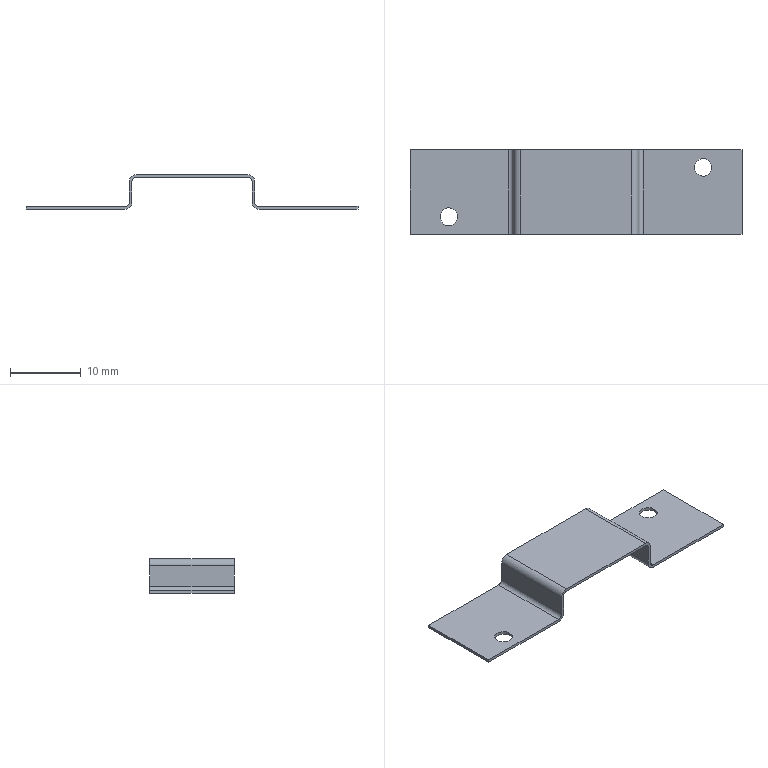Part | STEP file | ZXW722-L-04 | 1 solid | 26 faces | box 47 x 12 x 4.9 mm | volume 258.28 mm3 | plane 14 | cylinder 12 | commonest cylinder face diameters 1.2 x4 2 x4 2.5 x4
STEP:
#1=CARTESIAN_POINT('',(0.,0.,0.));
#2=DIRECTION('',(0.,0.,1.));
#3=DIRECTION('',(1.,0.,0.));
#4=AXIS2_PLACEMENT_3D('',#1,#2,#3);
#5=CARTESIAN_POINT('',(9.5,337.,-447.6));
#6=VERTEX_POINT('',#5);
#7=CARTESIAN_POINT('',(9.5,349.,-447.6));
#8=VERTEX_POINT('',#7);
#9=CARTESIAN_POINT('',(9.5,337.,-447.6));
#10=DIRECTION('',(0.,1.,0.));
#11=VECTOR('',#10,12.);
#12=LINE('',#9,#11);
#13=EDGE_CURVE('',#6,#8,#12,.T.);
#14=ORIENTED_EDGE('',*,*,#13,.F.);
#15=CARTESIAN_POINT('',(23.5,337.,-447.6));
#16=VERTEX_POINT('',#15);
#17=CARTESIAN_POINT('',(9.5,337.,-447.6));
#18=DIRECTION('',(1.,0.,0.));
#19=VECTOR('',#18,14.);
#20=LINE('',#17,#19);
#21=EDGE_CURVE('',#6,#16,#20,.T.);
#22=ORIENTED_EDGE('',*,*,#21,.T.);
#23=CARTESIAN_POINT('',(23.5,349.,-447.6));
#24=VERTEX_POINT('',#23);
#25=CARTESIAN_POINT('',(23.5,337.,-447.6));
#26=DIRECTION('',(0.,1.,0.));
#27=VECTOR('',#26,12.);
#28=LINE('',#25,#27);
#29=EDGE_CURVE('',#16,#24,#28,.T.);
#30=ORIENTED_EDGE('',*,*,#29,.T.);
#31=CARTESIAN_POINT('',(23.5,349.,-447.6));
#32=DIRECTION('',(-1.,0.,0.));
#33=VECTOR('',#32,14.);
#34=LINE('',#31,#33);
#35=EDGE_CURVE('',#24,#8,#34,.T.);
#36=ORIENTED_EDGE('',*,*,#35,.T.);
#37=EDGE_LOOP('',(#14,#22,#30,#36));
#38=FACE_OUTER_BOUND('',#37,.F.);
#39=CARTESIAN_POINT('',(19.25,346.5,-447.6));
#40=VERTEX_POINT('',#39);
#41=CARTESIAN_POINT('',(16.75,346.5,-447.6));
#42=VERTEX_POINT('',#41);
#43=CARTESIAN_POINT('',(18.,346.5,-447.6));
#44=DIRECTION('',(0.,0.,1.));
#45=DIRECTION('',(1.,0.,0.));
#46=AXIS2_PLACEMENT_3D('',#43,#44,#45);
#47=CIRCLE('',#46,1.25);
#48=EDGE_CURVE('',#40,#42,#47,.T.);
#49=ORIENTED_EDGE('',*,*,#48,.F.);
#50=CARTESIAN_POINT('',(18.,346.5,-447.6));
#51=DIRECTION('',(0.,0.,1.));
#52=DIRECTION('',(-1.,0.,0.));
#53=AXIS2_PLACEMENT_3D('',#50,#51,#52);
#54=CIRCLE('',#53,1.25);
#55=EDGE_CURVE('',#42,#40,#54,.T.);
#56=ORIENTED_EDGE('',*,*,#55,.F.);
#57=EDGE_LOOP('',(#49,#56));
#58=FACE_BOUND('',#57,.F.);
#59=CARTESIAN_POINT('',(0.,220.2,-447.6));
#60=DIRECTION('',(0.,0.,1.));
#61=DIRECTION('',(1.,0.,0.));
#62=AXIS2_PLACEMENT_3D('',#59,#60,#61);
#63=PLANE('',#62);
#64=ADVANCED_FACE('',(#38,#58),#63,.F.);
#65=CARTESIAN_POINT('',(-9.5,349.,-447.6));
#66=VERTEX_POINT('',#65);
#67=CARTESIAN_POINT('',(-9.5,337.,-447.6));
#68=VERTEX_POINT('',#67);
#69=CARTESIAN_POINT('',(-9.5,349.,-447.6));
#70=DIRECTION('',(0.,-1.,0.));
#71=VECTOR('',#70,12.);
#72=LINE('',#69,#71);
#73=EDGE_CURVE('',#66,#68,#72,.T.);
#74=ORIENTED_EDGE('',*,*,#73,.F.);
#75=CARTESIAN_POINT('',(-23.5,349.,-447.6));
#76=VERTEX_POINT('',#75);
#77=CARTESIAN_POINT('',(-9.5,349.,-447.6));
#78=DIRECTION('',(-1.,0.,0.));
#79=VECTOR('',#78,14.);
#80=LINE('',#77,#79);
#81=EDGE_CURVE('',#66,#76,#80,.T.);
#82=ORIENTED_EDGE('',*,*,#81,.T.);
#83=CARTESIAN_POINT('',(-23.5,337.,-447.6));
#84=VERTEX_POINT('',#83);
#85=CARTESIAN_POINT('',(-23.5,349.,-447.6));
#86=DIRECTION('',(0.,-1.,0.));
#87=VECTOR('',#86,12.);
#88=LINE('',#85,#87);
#89=EDGE_CURVE('',#76,#84,#88,.T.);
#90=ORIENTED_EDGE('',*,*,#89,.T.);
#91=CARTESIAN_POINT('',(-23.5,337.,-447.6));
#92=DIRECTION('',(1.,0.,0.));
#93=VECTOR('',#92,14.);
#94=LINE('',#91,#93);
#95=EDGE_CURVE('',#84,#68,#94,.T.);
#96=ORIENTED_EDGE('',*,*,#95,.T.);
#97=EDGE_LOOP('',(#74,#82,#90,#96));
#98=FACE_OUTER_BOUND('',#97,.F.);
#99=CARTESIAN_POINT('',(-16.75,339.5,-447.6));
#100=VERTEX_POINT('',#99);
#101=CARTESIAN_POINT('',(-19.25,339.5,-447.6));
#102=VERTEX_POINT('',#101);
#103=CARTESIAN_POINT('',(-18.,339.5,-447.6));
#104=DIRECTION('',(0.,0.,1.));
#105=DIRECTION('',(1.,0.,0.));
#106=AXIS2_PLACEMENT_3D('',#103,#104,#105);
#107=CIRCLE('',#106,1.25);
#108=EDGE_CURVE('',#100,#102,#107,.T.);
#109=ORIENTED_EDGE('',*,*,#108,.F.);
#110=CARTESIAN_POINT('',(-18.,339.5,-447.6));
#111=DIRECTION('',(0.,0.,1.));
#112=DIRECTION('',(-1.,0.,0.));
#113=AXIS2_PLACEMENT_3D('',#110,#111,#112);
#114=CIRCLE('',#113,1.25);
#115=EDGE_CURVE('',#102,#100,#114,.T.);
#116=ORIENTED_EDGE('',*,*,#115,.F.);
#117=EDGE_LOOP('',(#109,#116));
#118=FACE_BOUND('',#117,.F.);
#119=CARTESIAN_POINT('',(0.,220.2,-447.6));
#120=DIRECTION('',(0.,0.,1.));
#121=DIRECTION('',(1.,0.,0.));
#122=AXIS2_PLACEMENT_3D('',#119,#120,#121);
#123=PLANE('',#122);
#124=ADVANCED_FACE('',(#98,#118),#123,.F.);
#125=CARTESIAN_POINT('',(8.5,349.,-446.6));
#126=VERTEX_POINT('',#125);
#127=CARTESIAN_POINT('',(9.5,349.,-446.6));
#128=DIRECTION('',(0.,1.,0.));
#129=DIRECTION('',(0.,0.,-1.));
#130=AXIS2_PLACEMENT_3D('',#127,#128,#129);
#131=CIRCLE('',#130,1.);
#132=EDGE_CURVE('',#8,#126,#131,.T.);
#133=ORIENTED_EDGE('',*,*,#132,.T.);
#134=CARTESIAN_POINT('',(8.5,337.,-446.6));
#135=VERTEX_POINT('',#134);
#136=CARTESIAN_POINT('',(8.5,337.,-446.6));
#137=DIRECTION('',(0.,1.,0.));
#138=VECTOR('',#137,12.);
#139=LINE('',#136,#138);
#140=EDGE_CURVE('',#135,#126,#139,.T.);
#141=ORIENTED_EDGE('',*,*,#140,.F.);
#142=CARTESIAN_POINT('',(9.5,337.,-446.6));
#143=DIRECTION('',(0.,-1.,0.));
#144=DIRECTION('',(-1.,0.,0.));
#145=AXIS2_PLACEMENT_3D('',#142,#143,#144);
#146=CIRCLE('',#145,1.);
#147=EDGE_CURVE('',#135,#6,#146,.T.);
#148=ORIENTED_EDGE('',*,*,#147,.T.);
#149=ORIENTED_EDGE('',*,*,#13,.T.);
#150=EDGE_LOOP('',(#133,#141,#148,#149));
#151=FACE_OUTER_BOUND('',#150,.F.);
#152=CARTESIAN_POINT('',(9.5,317.446,-446.6));
#153=DIRECTION('',(0.,1.,0.));
#154=DIRECTION('',(0.,0.,-1.));
#155=AXIS2_PLACEMENT_3D('',#152,#153,#154);
#156=CYLINDRICAL_SURFACE('',#155,1.);
#157=ADVANCED_FACE('',(#151),#156,.T.);
#158=ORIENTED_EDGE('',*,*,#132,.F.);
#159=ORIENTED_EDGE('',*,*,#35,.F.);
#160=CARTESIAN_POINT('',(23.5,349.,-447.2));
#161=VERTEX_POINT('',#160);
#162=CARTESIAN_POINT('',(23.5,349.,-447.6));
#163=DIRECTION('',(0.,0.,1.));
#164=VECTOR('',#163,0.4);
#165=LINE('',#162,#164);
#166=EDGE_CURVE('',#24,#161,#165,.T.);
#167=ORIENTED_EDGE('',*,*,#166,.T.);
#168=CARTESIAN_POINT('',(9.5,349.,-447.2));
#169=VERTEX_POINT('',#168);
#170=CARTESIAN_POINT('',(23.5,349.,-447.2));
#171=DIRECTION('',(-1.,0.,0.));
#172=VECTOR('',#171,14.);
#173=LINE('',#170,#172);
#174=EDGE_CURVE('',#161,#169,#173,.T.);
#175=ORIENTED_EDGE('',*,*,#174,.T.);
#176=CARTESIAN_POINT('',(8.9,349.,-446.6));
#177=VERTEX_POINT('',#176);
#178=CARTESIAN_POINT('',(9.5,349.,-446.6));
#179=DIRECTION('',(0.,-1.,0.));
#180=DIRECTION('',(-1.,0.,0.));
#181=AXIS2_PLACEMENT_3D('',#178,#179,#180);
#182=CIRCLE('',#181,0.6);
#183=EDGE_CURVE('',#177,#169,#182,.T.);
#184=ORIENTED_EDGE('',*,*,#183,.F.);
#185=CARTESIAN_POINT('',(8.9,349.,-443.7));
#186=VERTEX_POINT('',#185);
#187=CARTESIAN_POINT('',(8.9,349.,-446.6));
#188=DIRECTION('',(0.,0.,1.));
#189=VECTOR('',#188,2.9);
#190=LINE('',#187,#189);
#191=EDGE_CURVE('',#177,#186,#190,.T.);
#192=ORIENTED_EDGE('',*,*,#191,.T.);
#193=CARTESIAN_POINT('',(7.9,349.,-442.7));
#194=VERTEX_POINT('',#193);
#195=CARTESIAN_POINT('',(7.9,349.,-443.7));
#196=DIRECTION('',(0.,1.,0.));
#197=DIRECTION('',(0.,0.,1.));
#198=AXIS2_PLACEMENT_3D('',#195,#196,#197);
#199=CIRCLE('',#198,1.);
#200=EDGE_CURVE('',#194,#186,#199,.T.);
#201=ORIENTED_EDGE('',*,*,#200,.F.);
#202=CARTESIAN_POINT('',(-7.9,349.,-442.7));
#203=VERTEX_POINT('',#202);
#204=CARTESIAN_POINT('',(7.9,349.,-442.7));
#205=DIRECTION('',(-1.,0.,0.));
#206=VECTOR('',#205,15.8);
#207=LINE('',#204,#206);
#208=EDGE_CURVE('',#194,#203,#207,.T.);
#209=ORIENTED_EDGE('',*,*,#208,.T.);
#210=CARTESIAN_POINT('',(-8.9,349.,-443.7));
#211=VERTEX_POINT('',#210);
#212=CARTESIAN_POINT('',(-7.9,349.,-443.7));
#213=DIRECTION('',(0.,1.,0.));
#214=DIRECTION('',(-1.,0.,0.));
#215=AXIS2_PLACEMENT_3D('',#212,#213,#214);
#216=CIRCLE('',#215,1.);
#217=EDGE_CURVE('',#211,#203,#216,.T.);
#218=ORIENTED_EDGE('',*,*,#217,.F.);
#219=CARTESIAN_POINT('',(-8.9,349.,-446.6));
#220=VERTEX_POINT('',#219);
#221=CARTESIAN_POINT('',(-8.9,349.,-446.6));
#222=DIRECTION('',(0.,0.,1.));
#223=VECTOR('',#222,2.9);
#224=LINE('',#221,#223);
#225=EDGE_CURVE('',#220,#211,#224,.T.);
#226=ORIENTED_EDGE('',*,*,#225,.F.);
#227=CARTESIAN_POINT('',(-9.5,349.,-447.2));
#228=VERTEX_POINT('',#227);
#229=CARTESIAN_POINT('',(-9.5,349.,-446.6));
#230=DIRECTION('',(0.,-1.,0.));
#231=DIRECTION('',(0.,0.,-1.));
#232=AXIS2_PLACEMENT_3D('',#229,#230,#231);
#233=CIRCLE('',#232,0.6);
#234=EDGE_CURVE('',#228,#220,#233,.T.);
#235=ORIENTED_EDGE('',*,*,#234,.F.);
#236=CARTESIAN_POINT('',(-23.5,349.,-447.2));
#237=VERTEX_POINT('',#236);
#238=CARTESIAN_POINT('',(-9.5,349.,-447.2));
#239=DIRECTION('',(-1.,0.,0.));
#240=VECTOR('',#239,14.);
#241=LINE('',#238,#240);
#242=EDGE_CURVE('',#228,#237,#241,.T.);
#243=ORIENTED_EDGE('',*,*,#242,.T.);
#244=CARTESIAN_POINT('',(-23.5,349.,-447.6));
#245=DIRECTION('',(0.,0.,1.));
#246=VECTOR('',#245,0.4);
#247=LINE('',#244,#246);
#248=EDGE_CURVE('',#76,#237,#247,.T.);
#249=ORIENTED_EDGE('',*,*,#248,.F.);
#250=ORIENTED_EDGE('',*,*,#81,.F.);
#251=CARTESIAN_POINT('',(-8.5,349.,-446.6));
#252=VERTEX_POINT('',#251);
#253=CARTESIAN_POINT('',(-9.5,349.,-446.6));
#254=DIRECTION('',(0.,1.,0.));
#255=DIRECTION('',(1.,0.,0.));
#256=AXIS2_PLACEMENT_3D('',#253,#254,#255);
#257=CIRCLE('',#256,1.);
#258=EDGE_CURVE('',#252,#66,#257,.T.);
#259=ORIENTED_EDGE('',*,*,#258,.F.);
#260=CARTESIAN_POINT('',(-8.5,349.,-443.7));
#261=VERTEX_POINT('',#260);
#262=CARTESIAN_POINT('',(-8.5,349.,-443.7));
#263=DIRECTION('',(0.,0.,-1.));
#264=VECTOR('',#263,2.9);
#265=LINE('',#262,#264);
#266=EDGE_CURVE('',#261,#252,#265,.T.);
#267=ORIENTED_EDGE('',*,*,#266,.F.);
#268=CARTESIAN_POINT('',(-7.9,349.,-443.1));
#269=VERTEX_POINT('',#268);
#270=CARTESIAN_POINT('',(-7.9,349.,-443.7));
#271=DIRECTION('',(0.,-1.,0.));
#272=DIRECTION('',(0.,0.,1.));
#273=AXIS2_PLACEMENT_3D('',#270,#271,#272);
#274=CIRCLE('',#273,0.6);
#275=EDGE_CURVE('',#269,#261,#274,.T.);
#276=ORIENTED_EDGE('',*,*,#275,.F.);
#277=CARTESIAN_POINT('',(7.9,349.,-443.1));
#278=VERTEX_POINT('',#277);
#279=CARTESIAN_POINT('',(7.9,349.,-443.1));
#280=DIRECTION('',(-1.,0.,0.));
#281=VECTOR('',#280,15.8);
#282=LINE('',#279,#281);
#283=EDGE_CURVE('',#278,#269,#282,.T.);
#284=ORIENTED_EDGE('',*,*,#283,.F.);
#285=CARTESIAN_POINT('',(8.5,349.,-443.7));
#286=VERTEX_POINT('',#285);
#287=CARTESIAN_POINT('',(7.9,349.,-443.7));
#288=DIRECTION('',(0.,-1.,0.));
#289=DIRECTION('',(1.,0.,0.));
#290=AXIS2_PLACEMENT_3D('',#287,#288,#289);
#291=CIRCLE('',#290,0.6);
#292=EDGE_CURVE('',#286,#278,#291,.T.);
#293=ORIENTED_EDGE('',*,*,#292,.F.);
#294=CARTESIAN_POINT('',(8.5,349.,-443.7));
#295=DIRECTION('',(0.,0.,-1.));
#296=VECTOR('',#295,2.9);
#297=LINE('',#294,#296);
#298=EDGE_CURVE('',#286,#126,#297,.T.);
#299=ORIENTED_EDGE('',*,*,#298,.T.);
#300=EDGE_LOOP('',(#158,#159,#167,#175,#184,#192,#201,#209,#218,#226,#235,#243,#249,#250,#259,#267,#276,#284,#293,#299));
#301=FACE_OUTER_BOUND('',#300,.F.);
#302=CARTESIAN_POINT('',(-8.5,349.,-447.6));
#303=DIRECTION('',(0.,1.,0.));
#304=DIRECTION('',(-1.,0.,0.));
#305=AXIS2_PLACEMENT_3D('',#302,#303,#304);
#306=PLANE('',#305);
#307=ADVANCED_FACE('',(#301),#306,.T.);
#308=ORIENTED_EDGE('',*,*,#29,.F.);
#309=CARTESIAN_POINT('',(23.5,337.,-447.2));
#310=VERTEX_POINT('',#309);
#311=CARTESIAN_POINT('',(23.5,337.,-447.6));
#312=DIRECTION('',(0.,0.,1.));
#313=VECTOR('',#312,0.4);
#314=LINE('',#311,#313);
#315=EDGE_CURVE('',#16,#310,#314,.T.);
#316=ORIENTED_EDGE('',*,*,#315,.T.);
#317=CARTESIAN_POINT('',(23.5,337.,-447.2));
#318=DIRECTION('',(0.,1.,0.));
#319=VECTOR('',#318,12.);
#320=LINE('',#317,#319);
#321=EDGE_CURVE('',#310,#161,#320,.T.);
#322=ORIENTED_EDGE('',*,*,#321,.T.);
#323=ORIENTED_EDGE('',*,*,#166,.F.);
#324=EDGE_LOOP('',(#308,#316,#322,#323));
#325=FACE_OUTER_BOUND('',#324,.F.);
#326=CARTESIAN_POINT('',(23.5,337.,-447.6));
#327=DIRECTION('',(1.,0.,0.));
#328=DIRECTION('',(0.,1.,0.));
#329=AXIS2_PLACEMENT_3D('',#326,#327,#328);
#330=PLANE('',#329);
#331=ADVANCED_FACE('',(#325),#330,.T.);
#332=ORIENTED_EDGE('',*,*,#147,.F.);
#333=CARTESIAN_POINT('',(8.5,337.,-443.7));
#334=VERTEX_POINT('',#333);
#335=CARTESIAN_POINT('',(8.5,337.,-446.6));
#336=DIRECTION('',(0.,0.,1.));
#337=VECTOR('',#336,2.9);
#338=LINE('',#335,#337);
#339=EDGE_CURVE('',#135,#334,#338,.T.);
#340=ORIENTED_EDGE('',*,*,#339,.T.);
#341=CARTESIAN_POINT('',(7.9,337.,-443.1));
#342=VERTEX_POINT('',#341);
#343=CARTESIAN_POINT('',(7.9,337.,-443.7));
#344=DIRECTION('',(0.,1.,0.));
#345=DIRECTION('',(0.,0.,1.));
#346=AXIS2_PLACEMENT_3D('',#343,#344,#345);
#347=CIRCLE('',#346,0.6);
#348=EDGE_CURVE('',#342,#334,#347,.T.);
#349=ORIENTED_EDGE('',*,*,#348,.F.);
#350=CARTESIAN_POINT('',(-7.9,337.,-443.1));
#351=VERTEX_POINT('',#350);
#352=CARTESIAN_POINT('',(-7.9,337.,-443.1));
#353=DIRECTION('',(1.,0.,0.));
#354=VECTOR('',#353,15.8);
#355=LINE('',#352,#354);
#356=EDGE_CURVE('',#351,#342,#355,.T.);
#357=ORIENTED_EDGE('',*,*,#356,.F.);
#358=CARTESIAN_POINT('',(-8.5,337.,-443.7));
#359=VERTEX_POINT('',#358);
#360=CARTESIAN_POINT('',(-7.9,337.,-443.7));
#361=DIRECTION('',(0.,1.,0.));
#362=DIRECTION('',(-1.,0.,0.));
#363=AXIS2_PLACEMENT_3D('',#360,#361,#362);
#364=CIRCLE('',#363,0.6);
#365=EDGE_CURVE('',#359,#351,#364,.T.);
#366=ORIENTED_EDGE('',*,*,#365,.F.);
#367=CARTESIAN_POINT('',(-8.5,337.,-446.6));
#368=VERTEX_POINT('',#367);
#369=CARTESIAN_POINT('',(-8.5,337.,-446.6));
#370=DIRECTION('',(0.,0.,1.));
#371=VECTOR('',#370,2.9);
#372=LINE('',#369,#371);
#373=EDGE_CURVE('',#368,#359,#372,.T.);
#374=ORIENTED_EDGE('',*,*,#373,.F.);
#375=CARTESIAN_POINT('',(-9.5,337.,-446.6));
#376=DIRECTION('',(0.,-1.,0.));
#377=DIRECTION('',(0.,0.,-1.));
#378=AXIS2_PLACEMENT_3D('',#375,#376,#377);
#379=CIRCLE('',#378,1.);
#380=EDGE_CURVE('',#68,#368,#379,.T.);
#381=ORIENTED_EDGE('',*,*,#380,.F.);
#382=ORIENTED_EDGE('',*,*,#95,.F.);
#383=CARTESIAN_POINT('',(-23.5,337.,-447.2));
#384=VERTEX_POINT('',#383);
#385=CARTESIAN_POINT('',(-23.5,337.,-447.6));
#386=DIRECTION('',(0.,0.,1.));
#387=VECTOR('',#386,0.4);
#388=LINE('',#385,#387);
#389=EDGE_CURVE('',#84,#384,#388,.T.);
#390=ORIENTED_EDGE('',*,*,#389,.T.);
#391=CARTESIAN_POINT('',(-9.5,337.,-447.2));
#392=VERTEX_POINT('',#391);
#393=CARTESIAN_POINT('',(-23.5,337.,-447.2));
#394=DIRECTION('',(1.,0.,0.));
#395=VECTOR('',#394,14.);
#396=LINE('',#393,#395);
#397=EDGE_CURVE('',#384,#392,#396,.T.);
#398=ORIENTED_EDGE('',*,*,#397,.T.);
#399=CARTESIAN_POINT('',(-8.9,337.,-446.6));
#400=VERTEX_POINT('',#399);
#401=CARTESIAN_POINT('',(-9.5,337.,-446.6));
#402=DIRECTION('',(0.,1.,0.));
#403=DIRECTION('',(1.,0.,0.));
#404=AXIS2_PLACEMENT_3D('',#401,#402,#403);
#405=CIRCLE('',#404,0.6);
#406=EDGE_CURVE('',#400,#392,#405,.T.);
#407=ORIENTED_EDGE('',*,*,#406,.F.);
#408=CARTESIAN_POINT('',(-8.9,337.,-443.7));
#409=VERTEX_POINT('',#408);
#410=CARTESIAN_POINT('',(-8.9,337.,-446.6));
#411=DIRECTION('',(0.,0.,1.));
#412=VECTOR('',#411,2.9);
#413=LINE('',#410,#412);
#414=EDGE_CURVE('',#400,#409,#413,.T.);
#415=ORIENTED_EDGE('',*,*,#414,.T.);
#416=CARTESIAN_POINT('',(-7.9,337.,-442.7));
#417=VERTEX_POINT('',#416);
#418=CARTESIAN_POINT('',(-7.9,337.,-443.7));
#419=DIRECTION('',(0.,-1.,0.));
#420=DIRECTION('',(0.,0.,1.));
#421=AXIS2_PLACEMENT_3D('',#418,#419,#420);
#422=CIRCLE('',#421,1.);
#423=EDGE_CURVE('',#417,#409,#422,.T.);
#424=ORIENTED_EDGE('',*,*,#423,.F.);
#425=CARTESIAN_POINT('',(7.9,337.,-442.7));
#426=VERTEX_POINT('',#425);
#427=CARTESIAN_POINT('',(-7.9,337.,-442.7));
#428=DIRECTION('',(1.,0.,0.));
#429=VECTOR('',#428,15.8);
#430=LINE('',#427,#429);
#431=EDGE_CURVE('',#417,#426,#430,.T.);
#432=ORIENTED_EDGE('',*,*,#431,.T.);
#433=CARTESIAN_POINT('',(8.9,337.,-443.7));
#434=VERTEX_POINT('',#433);
#435=CARTESIAN_POINT('',(7.9,337.,-443.7));
#436=DIRECTION('',(0.,-1.,0.));
#437=DIRECTION('',(1.,0.,0.));
#438=AXIS2_PLACEMENT_3D('',#435,#436,#437);
#439=CIRCLE('',#438,1.);
#440=EDGE_CURVE('',#434,#426,#439,.T.);
#441=ORIENTED_EDGE('',*,*,#440,.F.);
#442=CARTESIAN_POINT('',(8.9,337.,-446.6));
#443=VERTEX_POINT('',#442);
#444=CARTESIAN_POINT('',(8.9,337.,-446.6));
#445=DIRECTION('',(0.,0.,1.));
#446=VECTOR('',#445,2.9);
#447=LINE('',#444,#446);
#448=EDGE_CURVE('',#443,#434,#447,.T.);
#449=ORIENTED_EDGE('',*,*,#448,.F.);
#450=CARTESIAN_POINT('',(9.5,337.,-447.2));
#451=VERTEX_POINT('',#450);
#452=CARTESIAN_POINT('',(9.5,337.,-446.6));
#453=DIRECTION('',(0.,1.,0.));
#454=DIRECTION('',(0.,0.,-1.));
#455=AXIS2_PLACEMENT_3D('',#452,#453,#454);
#456=CIRCLE('',#455,0.6);
#457=EDGE_CURVE('',#451,#443,#456,.T.);
#458=ORIENTED_EDGE('',*,*,#457,.F.);
#459=CARTESIAN_POINT('',(9.5,337.,-447.2));
#460=DIRECTION('',(1.,0.,0.));
#461=VECTOR('',#460,14.);
#462=LINE('',#459,#461);
#463=EDGE_CURVE('',#451,#310,#462,.T.);
#464=ORIENTED_EDGE('',*,*,#463,.T.);
#465=ORIENTED_EDGE('',*,*,#315,.F.);
#466=ORIENTED_EDGE('',*,*,#21,.F.);
#467=EDGE_LOOP('',(#332,#340,#349,#357,#366,#374,#381,#382,#390,#398,#407,#415,#424,#432,#441,#449,#458,#464,#465,#466));
#468=FACE_OUTER_BOUND('',#467,.F.);
#469=CARTESIAN_POINT('',(-20.5,337.,-447.6));
#470=DIRECTION('',(0.,-1.,0.));
#471=DIRECTION('',(1.,0.,0.));
#472=AXIS2_PLACEMENT_3D('',#469,#470,#471);
#473=PLANE('',#472);
#474=ADVANCED_FACE('',(#468),#473,.T.);
#475=ORIENTED_EDGE('',*,*,#140,.T.);
#476=ORIENTED_EDGE('',*,*,#298,.F.);
#477=CARTESIAN_POINT('',(8.5,349.,-443.7));
#478=DIRECTION('',(0.,-1.,0.));
#479=VECTOR('',#478,12.);
#480=LINE('',#477,#479);
#481=EDGE_CURVE('',#286,#334,#480,.T.);
#482=ORIENTED_EDGE('',*,*,#481,.T.);
#483=ORIENTED_EDGE('',*,*,#339,.F.);
#484=EDGE_LOOP('',(#475,#476,#482,#483));
#485=FACE_OUTER_BOUND('',#484,.F.);
#486=CARTESIAN_POINT('',(8.5,352.,-447.6));
#487=DIRECTION('',(-1.,0.,0.));
#488=DIRECTION('',(0.,-1.,0.));
#489=AXIS2_PLACEMENT_3D('',#486,#487,#488);
#490=PLANE('',#489);
#491=ADVANCED_FACE('',(#485),#490,.T.);
#492=ORIENTED_EDGE('',*,*,#481,.F.);
#493=ORIENTED_EDGE('',*,*,#292,.T.);
#494=CARTESIAN_POINT('',(7.9,349.,-443.1));
#495=DIRECTION('',(0.,-1.,0.));
#496=VECTOR('',#495,12.);
#497=LINE('',#494,#496);
#498=EDGE_CURVE('',#278,#342,#497,.T.);
#499=ORIENTED_EDGE('',*,*,#498,.T.);
#500=ORIENTED_EDGE('',*,*,#348,.T.);
#501=EDGE_LOOP('',(#492,#493,#499,#500));
#502=FACE_OUTER_BOUND('',#501,.F.);
#503=CARTESIAN_POINT('',(7.9,371.554,-443.7));
#504=DIRECTION('',(0.,-1.,0.));
#505=DIRECTION('',(1.,0.,0.));
#506=AXIS2_PLACEMENT_3D('',#503,#504,#505);
#507=CYLINDRICAL_SURFACE('',#506,0.6);
#508=ADVANCED_FACE('',(#502),#507,.F.);
#509=CARTESIAN_POINT('',(-7.9,337.,-443.1));
#510=DIRECTION('',(0.,1.,0.));
#511=VECTOR('',#510,12.);
#512=LINE('',#509,#511);
#513=EDGE_CURVE('',#351,#269,#512,.T.);
#514=ORIENTED_EDGE('',*,*,#513,.F.);
#515=ORIENTED_EDGE('',*,*,#356,.T.);
#516=ORIENTED_EDGE('',*,*,#498,.F.);
#517=ORIENTED_EDGE('',*,*,#283,.T.);
#518=EDGE_LOOP('',(#514,#515,#516,#517));
#519=FACE_OUTER_BOUND('',#518,.F.);
#520=CARTESIAN_POINT('',(0.,0.,-443.1));
#521=DIRECTION('',(0.,0.,1.));
#522=DIRECTION('',(1.,0.,0.));
#523=AXIS2_PLACEMENT_3D('',#520,#521,#522);
#524=PLANE('',#523);
#525=ADVANCED_FACE('',(#519),#524,.F.);
#526=CARTESIAN_POINT('',(-8.5,337.,-443.7));
#527=DIRECTION('',(0.,1.,0.));
#528=VECTOR('',#527,12.);
#529=LINE('',#526,#528);
#530=EDGE_CURVE('',#359,#261,#529,.T.);
#531=ORIENTED_EDGE('',*,*,#530,.F.);
#532=ORIENTED_EDGE('',*,*,#365,.T.);
#533=ORIENTED_EDGE('',*,*,#513,.T.);
#534=ORIENTED_EDGE('',*,*,#275,.T.);
#535=EDGE_LOOP('',(#531,#532,#533,#534));
#536=FACE_OUTER_BOUND('',#535,.F.);
#537=CARTESIAN_POINT('',(-7.9,317.446,-443.7));
#538=DIRECTION('',(0.,1.,0.));
#539=DIRECTION('',(-1.,0.,0.));
#540=AXIS2_PLACEMENT_3D('',#537,#538,#539);
#541=CYLINDRICAL_SURFACE('',#540,0.6);
#542=ADVANCED_FACE('',(#536),#541,.F.);
#543=CARTESIAN_POINT('',(-8.5,349.,-446.6));
#544=DIRECTION('',(0.,-1.,0.));
#545=VECTOR('',#544,12.);
#546=LINE('',#543,#545);
#547=EDGE_CURVE('',#252,#368,#546,.T.);
#548=ORIENTED_EDGE('',*,*,#547,.T.);
#549=ORIENTED_EDGE('',*,*,#373,.T.);
#550=ORIENTED_EDGE('',*,*,#530,.T.);
#551=ORIENTED_EDGE('',*,*,#266,.T.);
#552=EDGE_LOOP('',(#548,#549,#550,#551));
#553=FACE_OUTER_BOUND('',#552,.F.);
#554=CARTESIAN_POINT('',(-8.5,337.,-447.6));
#555=DIRECTION('',(1.,0.,0.));
#556=DIRECTION('',(0.,1.,0.));
#557=AXIS2_PLACEMENT_3D('',#554,#555,#556);
#558=PLANE('',#557);
#559=ADVANCED_FACE('',(#553),#558,.T.);
#560=ORIENTED_EDGE('',*,*,#380,.T.);
#561=ORIENTED_EDGE('',*,*,#547,.F.);
#562=ORIENTED_EDGE('',*,*,#258,.T.);
#563=ORIENTED_EDGE('',*,*,#73,.T.);
#564=EDGE_LOOP('',(#560,#561,#562,#563));
#565=FACE_OUTER_BOUND('',#564,.F.);
#566=CARTESIAN_POINT('',(-9.5,371.554,-446.6));
#567=DIRECTION('',(0.,-1.,0.));
#568=DIRECTION('',(0.,0.,-1.));
#569=AXIS2_PLACEMENT_3D('',#566,#567,#568);
#570=CYLINDRICAL_SURFACE('',#569,1.);
#571=ADVANCED_FACE('',(#565),#570,.T.);
#572=ORIENTED_EDGE('',*,*,#89,.F.);
#573=ORIENTED_EDGE('',*,*,#248,.T.);
#574=CARTESIAN_POINT('',(-23.5,349.,-447.2));
#575=DIRECTION('',(0.,-1.,0.));
#576=VECTOR('',#575,12.);
#577=LINE('',#574,#576);
#578=EDGE_CURVE('',#237,#384,#577,.T.);
#579=ORIENTED_EDGE('',*,*,#578,.T.);
#580=ORIENTED_EDGE('',*,*,#389,.F.);
#581=EDGE_LOOP('',(#572,#573,#579,#580));
#582=FACE_OUTER_BOUND('',#581,.F.);
#583=CARTESIAN_POINT('',(-23.5,352.,-447.6));
#584=DIRECTION('',(-1.,0.,0.));
#585=DIRECTION('',(0.,-1.,0.));
#586=AXIS2_PLACEMENT_3D('',#583,#584,#585);
#587=PLANE('',#586);
#588=ADVANCED_FACE('',(#582),#587,.T.);
#589=CARTESIAN_POINT('',(9.5,337.,-447.2));
#590=DIRECTION('',(0.,1.,0.));
#591=VECTOR('',#590,12.);
#592=LINE('',#589,#591);
#593=EDGE_CURVE('',#451,#169,#592,.T.);
#594=ORIENTED_EDGE('',*,*,#593,.T.);
#595=ORIENTED_EDGE('',*,*,#174,.F.);
#596=ORIENTED_EDGE('',*,*,#321,.F.);
#597=ORIENTED_EDGE('',*,*,#463,.F.);
#598=EDGE_LOOP('',(#594,#595,#596,#597));
#599=FACE_OUTER_BOUND('',#598,.F.);
#600=CARTESIAN_POINT('',(19.25,346.5,-447.2));
#601=VERTEX_POINT('',#600);
#602=CARTESIAN_POINT('',(16.75,346.5,-447.2));
#603=VERTEX_POINT('',#602);
#604=CARTESIAN_POINT('',(18.,346.5,-447.2));
#605=DIRECTION('',(0.,0.,1.));
#606=DIRECTION('',(1.,0.,0.));
#607=AXIS2_PLACEMENT_3D('',#604,#605,#606);
#608=CIRCLE('',#607,1.25);
#609=EDGE_CURVE('',#601,#603,#608,.T.);
#610=ORIENTED_EDGE('',*,*,#609,.T.);
#611=CARTESIAN_POINT('',(18.,346.5,-447.2));
#612=DIRECTION('',(0.,0.,1.));
#613=DIRECTION('',(-1.,0.,0.));
#614=AXIS2_PLACEMENT_3D('',#611,#612,#613);
#615=CIRCLE('',#614,1.25);
#616=EDGE_CURVE('',#603,#601,#615,.T.);
#617=ORIENTED_EDGE('',*,*,#616,.T.);
#618=EDGE_LOOP('',(#610,#617));
#619=FACE_BOUND('',#618,.F.);
#620=CARTESIAN_POINT('',(0.,220.2,-447.2));
#621=DIRECTION('',(0.,0.,1.));
#622=DIRECTION('',(1.,0.,0.));
#623=AXIS2_PLACEMENT_3D('',#620,#621,#622);
#624=PLANE('',#623);
#625=ADVANCED_FACE('',(#599,#619),#624,.T.);
#626=CARTESIAN_POINT('',(-9.5,349.,-447.2));
#627=DIRECTION('',(0.,-1.,0.));
#628=VECTOR('',#627,12.);
#629=LINE('',#626,#628);
#630=EDGE_CURVE('',#228,#392,#629,.T.);
#631=ORIENTED_EDGE('',*,*,#630,.T.);
#632=ORIENTED_EDGE('',*,*,#397,.F.);
#633=ORIENTED_EDGE('',*,*,#578,.F.);
#634=ORIENTED_EDGE('',*,*,#242,.F.);
#635=EDGE_LOOP('',(#631,#632,#633,#634));
#636=FACE_OUTER_BOUND('',#635,.F.);
#637=CARTESIAN_POINT('',(-16.75,339.5,-447.2));
#638=VERTEX_POINT('',#637);
#639=CARTESIAN_POINT('',(-19.25,339.5,-447.2));
#640=VERTEX_POINT('',#639);
#641=CARTESIAN_POINT('',(-18.,339.5,-447.2));
#642=DIRECTION('',(0.,0.,1.));
#643=DIRECTION('',(1.,0.,0.));
#644=AXIS2_PLACEMENT_3D('',#641,#642,#643);
#645=CIRCLE('',#644,1.25);
#646=EDGE_CURVE('',#638,#640,#645,.T.);
#647=ORIENTED_EDGE('',*,*,#646,.T.);
#648=CARTESIAN_POINT('',(-18.,339.5,-447.2));
#649=DIRECTION('',(0.,0.,1.));
#650=DIRECTION('',(-1.,0.,0.));
#651=AXIS2_PLACEMENT_3D('',#648,#649,#650);
#652=CIRCLE('',#651,1.25);
#653=EDGE_CURVE('',#640,#638,#652,.T.);
#654=ORIENTED_EDGE('',*,*,#653,.T.);
#655=EDGE_LOOP('',(#647,#654));
#656=FACE_BOUND('',#655,.F.);
#657=CARTESIAN_POINT('',(0.,220.2,-447.2));
#658=DIRECTION('',(0.,0.,1.));
#659=DIRECTION('',(1.,0.,0.));
#660=AXIS2_PLACEMENT_3D('',#657,#658,#659);
#661=PLANE('',#660);
#662=ADVANCED_FACE('',(#636,#656),#661,.T.);
#663=ORIENTED_EDGE('',*,*,#593,.F.);
#664=ORIENTED_EDGE('',*,*,#457,.T.);
#665=CARTESIAN_POINT('',(8.9,337.,-446.6));
#666=DIRECTION('',(0.,1.,0.));
#667=VECTOR('',#666,12.);
#668=LINE('',#665,#667);
#669=EDGE_CURVE('',#443,#177,#668,.T.);
#670=ORIENTED_EDGE('',*,*,#669,.T.);
#671=ORIENTED_EDGE('',*,*,#183,.T.);
#672=EDGE_LOOP('',(#663,#664,#670,#671));
#673=FACE_OUTER_BOUND('',#672,.F.);
#674=CARTESIAN_POINT('',(9.5,317.446,-446.6));
#675=DIRECTION('',(0.,1.,0.));
#676=DIRECTION('',(0.,0.,-1.));
#677=AXIS2_PLACEMENT_3D('',#674,#675,#676);
#678=CYLINDRICAL_SURFACE('',#677,0.6);
#679=ADVANCED_FACE('',(#673),#678,.F.);
#680=CARTESIAN_POINT('',(8.9,337.,-443.7));
#681=DIRECTION('',(0.,1.,0.));
#682=VECTOR('',#681,12.);
#683=LINE('',#680,#682);
#684=EDGE_CURVE('',#434,#186,#683,.T.);
#685=ORIENTED_EDGE('',*,*,#684,.T.);
#686=ORIENTED_EDGE('',*,*,#191,.F.);
#687=ORIENTED_EDGE('',*,*,#669,.F.);
#688=ORIENTED_EDGE('',*,*,#448,.T.);
#689=EDGE_LOOP('',(#685,#686,#687,#688));
#690=FACE_OUTER_BOUND('',#689,.F.);
#691=CARTESIAN_POINT('',(8.9,337.,-447.2));
#692=DIRECTION('',(1.,0.,0.));
#693=DIRECTION('',(0.,1.,0.));
#694=AXIS2_PLACEMENT_3D('',#691,#692,#693);
#695=PLANE('',#694);
#696=ADVANCED_FACE('',(#690),#695,.T.);
#697=ORIENTED_EDGE('',*,*,#200,.T.);
#698=ORIENTED_EDGE('',*,*,#684,.F.);
#699=ORIENTED_EDGE('',*,*,#440,.T.);
#700=CARTESIAN_POINT('',(7.9,337.,-442.7));
#701=DIRECTION('',(0.,1.,0.));
#702=VECTOR('',#701,12.);
#703=LINE('',#700,#702);
#704=EDGE_CURVE('',#426,#194,#703,.T.);
#705=ORIENTED_EDGE('',*,*,#704,.T.);
#706=EDGE_LOOP('',(#697,#698,#699,#705));
#707=FACE_OUTER_BOUND('',#706,.F.);
#708=CARTESIAN_POINT('',(7.9,317.446,-443.7));
#709=DIRECTION('',(0.,1.,0.));
#710=DIRECTION('',(0.,0.,1.));
#711=AXIS2_PLACEMENT_3D('',#708,#709,#710);
#712=CYLINDRICAL_SURFACE('',#711,1.);
#713=ADVANCED_FACE('',(#707),#712,.T.);
#714=ORIENTED_EDGE('',*,*,#704,.F.);
#715=ORIENTED_EDGE('',*,*,#431,.F.);
#716=CARTESIAN_POINT('',(-7.9,349.,-442.7));
#717=DIRECTION('',(0.,-1.,0.));
#718=VECTOR('',#717,12.);
#719=LINE('',#716,#718);
#720=EDGE_CURVE('',#203,#417,#719,.T.);
#721=ORIENTED_EDGE('',*,*,#720,.F.);
#722=ORIENTED_EDGE('',*,*,#208,.F.);
#723=EDGE_LOOP('',(#714,#715,#721,#722));
#724=FACE_OUTER_BOUND('',#723,.F.);
#725=CARTESIAN_POINT('',(0.,0.,-442.7));
#726=DIRECTION('',(0.,0.,1.));
#727=DIRECTION('',(1.,0.,0.));
#728=AXIS2_PLACEMENT_3D('',#725,#726,#727);
#729=PLANE('',#728);
#730=ADVANCED_FACE('',(#724),#729,.T.);
#731=ORIENTED_EDGE('',*,*,#423,.T.);
#732=CARTESIAN_POINT('',(-8.9,349.,-443.7));
#733=DIRECTION('',(0.,-1.,0.));
#734=VECTOR('',#733,12.);
#735=LINE('',#732,#734);
#736=EDGE_CURVE('',#211,#409,#735,.T.);
#737=ORIENTED_EDGE('',*,*,#736,.F.);
#738=ORIENTED_EDGE('',*,*,#217,.T.);
#739=ORIENTED_EDGE('',*,*,#720,.T.);
#740=EDGE_LOOP('',(#731,#737,#738,#739));
#741=FACE_OUTER_BOUND('',#740,.F.);
#742=CARTESIAN_POINT('',(-7.9,371.554,-443.7));
#743=DIRECTION('',(0.,-1.,0.));
#744=DIRECTION('',(0.,0.,1.));
#745=AXIS2_PLACEMENT_3D('',#742,#743,#744);
#746=CYLINDRICAL_SURFACE('',#745,1.);
#747=ADVANCED_FACE('',(#741),#746,.T.);
#748=ORIENTED_EDGE('',*,*,#736,.T.);
#749=ORIENTED_EDGE('',*,*,#414,.F.);
#750=CARTESIAN_POINT('',(-8.9,349.,-446.6));
#751=DIRECTION('',(0.,-1.,0.));
#752=VECTOR('',#751,12.);
#753=LINE('',#750,#752);
#754=EDGE_CURVE('',#220,#400,#753,.T.);
#755=ORIENTED_EDGE('',*,*,#754,.F.);
#756=ORIENTED_EDGE('',*,*,#225,.T.);
#757=EDGE_LOOP('',(#748,#749,#755,#756));
#758=FACE_OUTER_BOUND('',#757,.F.);
#759=CARTESIAN_POINT('',(-8.9,352.,-447.2));
#760=DIRECTION('',(-1.,0.,0.));
#761=DIRECTION('',(0.,-1.,0.));
#762=AXIS2_PLACEMENT_3D('',#759,#760,#761);
#763=PLANE('',#762);
#764=ADVANCED_FACE('',(#758),#763,.T.);
#765=ORIENTED_EDGE('',*,*,#630,.F.);
#766=ORIENTED_EDGE('',*,*,#234,.T.);
#767=ORIENTED_EDGE('',*,*,#754,.T.);
#768=ORIENTED_EDGE('',*,*,#406,.T.);
#769=EDGE_LOOP('',(#765,#766,#767,#768));
#770=FACE_OUTER_BOUND('',#769,.F.);
#771=CARTESIAN_POINT('',(-9.5,371.554,-446.6));
#772=DIRECTION('',(0.,-1.,0.));
#773=DIRECTION('',(0.,0.,-1.));
#774=AXIS2_PLACEMENT_3D('',#771,#772,#773);
#775=CYLINDRICAL_SURFACE('',#774,0.6);
#776=ADVANCED_FACE('',(#770),#775,.F.);
#777=ORIENTED_EDGE('',*,*,#48,.T.);
#778=CARTESIAN_POINT('',(16.75,346.5,-447.6));
#779=DIRECTION('',(0.,0.,1.));
#780=VECTOR('',#779,0.4);
#781=LINE('',#778,#780);
#782=EDGE_CURVE('',#42,#603,#781,.T.);
#783=ORIENTED_EDGE('',*,*,#782,.T.);
#784=ORIENTED_EDGE('',*,*,#609,.F.);
#785=CARTESIAN_POINT('',(19.25,346.5,-447.6));
#786=DIRECTION('',(0.,0.,1.));
#787=VECTOR('',#786,0.4);
#788=LINE('',#785,#787);
#789=EDGE_CURVE('',#40,#601,#788,.T.);
#790=ORIENTED_EDGE('',*,*,#789,.F.);
#791=EDGE_LOOP('',(#777,#783,#784,#790));
#792=FACE_OUTER_BOUND('',#791,.F.);
#793=CARTESIAN_POINT('',(18.,346.5,-452.575));
#794=DIRECTION('',(0.,0.,1.));
#795=DIRECTION('',(1.,0.,0.));
#796=AXIS2_PLACEMENT_3D('',#793,#794,#795);
#797=CYLINDRICAL_SURFACE('',#796,1.25);
#798=ADVANCED_FACE('',(#792),#797,.F.);
#799=ORIENTED_EDGE('',*,*,#55,.T.);
#800=ORIENTED_EDGE('',*,*,#789,.T.);
#801=ORIENTED_EDGE('',*,*,#616,.F.);
#802=ORIENTED_EDGE('',*,*,#782,.F.);
#803=EDGE_LOOP('',(#799,#800,#801,#802));
#804=FACE_OUTER_BOUND('',#803,.F.);
#805=CARTESIAN_POINT('',(18.,346.5,-452.575));
#806=DIRECTION('',(0.,0.,1.));
#807=DIRECTION('',(1.,0.,0.));
#808=AXIS2_PLACEMENT_3D('',#805,#806,#807);
#809=CYLINDRICAL_SURFACE('',#808,1.25);
#810=ADVANCED_FACE('',(#804),#809,.F.);
#811=ORIENTED_EDGE('',*,*,#108,.T.);
#812=CARTESIAN_POINT('',(-19.25,339.5,-447.6));
#813=DIRECTION('',(0.,0.,1.));
#814=VECTOR('',#813,0.4);
#815=LINE('',#812,#814);
#816=EDGE_CURVE('',#102,#640,#815,.T.);
#817=ORIENTED_EDGE('',*,*,#816,.T.);
#818=ORIENTED_EDGE('',*,*,#646,.F.);
#819=CARTESIAN_POINT('',(-16.75,339.5,-447.6));
#820=DIRECTION('',(0.,0.,1.));
#821=VECTOR('',#820,0.4);
#822=LINE('',#819,#821);
#823=EDGE_CURVE('',#100,#638,#822,.T.);
#824=ORIENTED_EDGE('',*,*,#823,.F.);
#825=EDGE_LOOP('',(#811,#817,#818,#824));
#826=FACE_OUTER_BOUND('',#825,.F.);
#827=CARTESIAN_POINT('',(-18.,339.5,-452.575));
#828=DIRECTION('',(0.,0.,1.));
#829=DIRECTION('',(1.,0.,0.));
#830=AXIS2_PLACEMENT_3D('',#827,#828,#829);
#831=CYLINDRICAL_SURFACE('',#830,1.25);
#832=ADVANCED_FACE('',(#826),#831,.F.);
#833=ORIENTED_EDGE('',*,*,#115,.T.);
#834=ORIENTED_EDGE('',*,*,#823,.T.);
#835=ORIENTED_EDGE('',*,*,#653,.F.);
#836=ORIENTED_EDGE('',*,*,#816,.F.);
#837=EDGE_LOOP('',(#833,#834,#835,#836));
#838=FACE_OUTER_BOUND('',#837,.F.);
#839=CARTESIAN_POINT('',(-18.,339.5,-452.575));
#840=DIRECTION('',(0.,0.,1.));
#841=DIRECTION('',(1.,0.,0.));
#842=AXIS2_PLACEMENT_3D('',#839,#840,#841);
#843=CYLINDRICAL_SURFACE('',#842,1.25);
#844=ADVANCED_FACE('',(#838),#843,.F.);
#845=CLOSED_SHELL('',(#64,#124,#157,#307,#331,#474,#491,#508,#525,#542,#559,#571,#588,#625,#662,#679,#696,#713,#730,#747,#764,#776,#798,#810,#832,#844));
#846=MANIFOLD_SOLID_BREP('',#845);
#847=(LENGTH_UNIT()NAMED_UNIT(*)SI_UNIT(.MILLI.,.METRE.));
#848=UNCERTAINTY_MEASURE_WITH_UNIT(LENGTH_MEASURE(0.009512),#847,'','');
#849=(NAMED_UNIT(*)PLANE_ANGLE_UNIT()SI_UNIT($,.RADIAN.));
#850=PLANE_ANGLE_MEASURE_WITH_UNIT(PLANE_ANGLE_MEASURE(0.01745),#849);
#851=(CONVERSION_BASED_UNIT('DEGREE',#850)NAMED_UNIT(*)PLANE_ANGLE_UNIT());
#852=(NAMED_UNIT(*)SI_UNIT($,.STERADIAN.)SOLID_ANGLE_UNIT());
#853=(GEOMETRIC_REPRESENTATION_CONTEXT(3)GLOBAL_UNCERTAINTY_ASSIGNED_CONTEXT((#848))GLOBAL_UNIT_ASSIGNED_CONTEXT((#847,#851,#852))REPRESENTATION_CONTEXT('',''));
#854=ADVANCED_BREP_SHAPE_REPRESENTATION('',(#4,#846),#853);